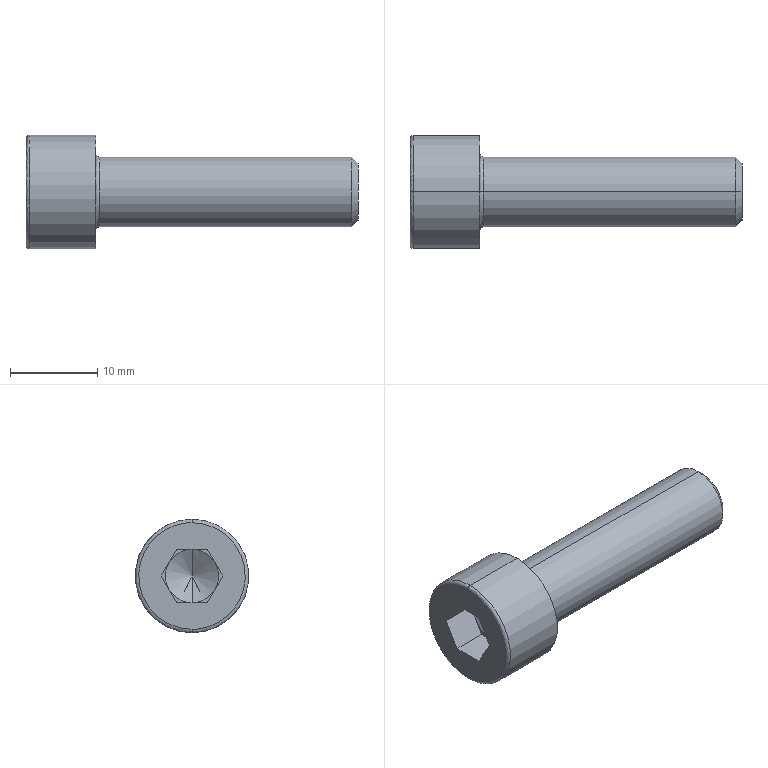Part | SolidWorks | features BaseBody 1 | 1 solid | 27 faces | box 38 x 13 x 13 mm | volume 2418 mm3 | plane 15 | spline 4 | cylinder 4 | cone 4 | commonest cylinder face diameters 8 x2 13 x2
STEP:
#1=CARTESIAN_POINT('',(8.,0.,4.4));
#2=VERTEX_POINT('',#1);
#3=CARTESIAN_POINT('',(8.,0.,-4.4));
#4=VERTEX_POINT('',#3);
#5=CARTESIAN_POINT('',(8.,0.,4.4));
#6=CARTESIAN_POINT('',(8.,0.2797,4.4));
#7=CARTESIAN_POINT('',(8.,0.6919,4.361));
#8=CARTESIAN_POINT('',(8.,1.16,4.249));
#9=CARTESIAN_POINT('',(8.,1.391,4.176));
#10=CARTESIAN_POINT('',(8.,1.489,4.141));
#11=CARTESIAN_POINT('',(8.,1.554,4.116));
#12=CARTESIAN_POINT('',(8.,1.585,4.105));
#13=CARTESIAN_POINT('',(8.,1.758,4.036));
#14=CARTESIAN_POINT('',(8.,1.96,3.944));
#15=CARTESIAN_POINT('',(8.,2.154,3.837));
#16=CARTESIAN_POINT('',(8.,2.282,3.763));
#17=CARTESIAN_POINT('',(8.,2.344,3.724));
#18=CARTESIAN_POINT('',(8.,2.662,3.517));
#19=CARTESIAN_POINT('',(8.,2.897,3.326));
#20=CARTESIAN_POINT('',(8.,3.219,3.004));
#21=CARTESIAN_POINT('',(8.,3.37,2.836));
#22=CARTESIAN_POINT('',(8.,3.509,2.656));
#23=CARTESIAN_POINT('',(8.,3.598,2.534));
#24=CARTESIAN_POINT('',(8.,3.642,2.47));
#25=CARTESIAN_POINT('',(8.,3.764,2.283));
#26=CARTESIAN_POINT('',(8.,3.876,2.092));
#27=CARTESIAN_POINT('',(8.,3.989,1.859));
#28=CARTESIAN_POINT('',(8.,4.042,1.74));
#29=CARTESIAN_POINT('',(8.,4.063,1.689));
#30=CARTESIAN_POINT('',(8.,4.077,1.654));
#31=CARTESIAN_POINT('',(8.,4.085,1.636));
#32=CARTESIAN_POINT('',(8.,4.297,1.1));
#33=CARTESIAN_POINT('',(8.,4.4,0.5592));
#34=CARTESIAN_POINT('',(8.,4.4,-0.2796));
#35=CARTESIAN_POINT('',(8.,4.361,-0.6917));
#36=CARTESIAN_POINT('',(8.,4.249,-1.16));
#37=CARTESIAN_POINT('',(8.,4.176,-1.391));
#38=CARTESIAN_POINT('',(8.,4.141,-1.489));
#39=CARTESIAN_POINT('',(8.,4.116,-1.554));
#40=CARTESIAN_POINT('',(8.,4.105,-1.585));
#41=CARTESIAN_POINT('',(8.,4.036,-1.758));
#42=CARTESIAN_POINT('',(8.,3.944,-1.96));
#43=CARTESIAN_POINT('',(8.,3.837,-2.154));
#44=CARTESIAN_POINT('',(8.,3.763,-2.282));
#45=CARTESIAN_POINT('',(8.,3.724,-2.344));
#46=CARTESIAN_POINT('',(8.,3.517,-2.662));
#47=CARTESIAN_POINT('',(8.,3.326,-2.897));
#48=CARTESIAN_POINT('',(8.,3.004,-3.219));
#49=CARTESIAN_POINT('',(8.,2.836,-3.37));
#50=CARTESIAN_POINT('',(8.,2.656,-3.509));
#51=CARTESIAN_POINT('',(8.,2.534,-3.598));
#52=CARTESIAN_POINT('',(8.,2.47,-3.642));
#53=CARTESIAN_POINT('',(8.,2.283,-3.764));
#54=CARTESIAN_POINT('',(8.,2.092,-3.876));
#55=CARTESIAN_POINT('',(8.,1.859,-3.989));
#56=CARTESIAN_POINT('',(8.,1.74,-4.042));
#57=CARTESIAN_POINT('',(8.,1.689,-4.063));
#58=CARTESIAN_POINT('',(8.,1.654,-4.077));
#59=CARTESIAN_POINT('',(8.,1.636,-4.085));
#60=CARTESIAN_POINT('',(8.,1.1,-4.297));
#61=CARTESIAN_POINT('',(8.,0.5597,-4.4));
#62=CARTESIAN_POINT('',(8.,0.,-4.4));
#63=B_SPLINE_CURVE_WITH_KNOTS('',3,(#5,#6,#7,#8,#9,#10,#11,#12,#13,#14,#15,#16,#17,#18,#19,#20,#21,#22,#23,#24,#25,#26,#27,#28,#29,#30,#31,#32,#33,#34,#35,#36,#37,#38,#39,#40,#41,#42,#43,#44,#45,#46,#47,#48,#49,#50,#51,#52,#53,#54,#55,#56,#57,#58,#59,#60,#61,#62),.UNSPECIFIED.,.F.,.F.,(4,1,1,1,2,2,1,2,2,2,1,2,2,1,1,1,2,2,2,1,1,1,2,2,1,2,2,2,1,2,2,1,1,1,2,2,4),(0.,0.0625,0.09375,0.1094,0.1172,0.125,0.1563,0.1719,0.1875,0.25,0.2813,0.2969,0.3125,0.3438,0.3594,0.3672,0.3711,0.375,0.5,0.5625,0.5938,0.6094,0.6172,0.625,0.6563,0.6719,0.6875,0.75,0.7813,0.7969,0.8125,0.8438,0.8594,0.8672,0.8711,0.875,1.),.UNSPECIFIED.);
#64=EDGE_CURVE('',#2,#4,#63,.T.);
#65=ORIENTED_EDGE('',*,*,#64,.F.);
#66=CARTESIAN_POINT('',(8.4,0.,4.));
#67=VERTEX_POINT('',#66);
#68=CARTESIAN_POINT('',(8.4,0.,4.4));
#69=DIRECTION('',(0.,-1.,0.));
#70=DIRECTION('',(0.,0.,1.));
#71=AXIS2_PLACEMENT_3D('',#68,#69,#70);
#72=CIRCLE('',#71,0.4);
#73=EDGE_CURVE('',#2,#67,#72,.T.);
#74=ORIENTED_EDGE('',*,*,#73,.T.);
#75=CARTESIAN_POINT('',(8.4,0.,-4.));
#76=VERTEX_POINT('',#75);
#77=CARTESIAN_POINT('',(8.4,0.,0.));
#78=DIRECTION('',(1.,0.,0.));
#79=DIRECTION('',(0.,0.,1.));
#80=AXIS2_PLACEMENT_3D('',#77,#78,#79);
#81=CIRCLE('',#80,4.);
#82=EDGE_CURVE('',#76,#67,#81,.T.);
#83=ORIENTED_EDGE('',*,*,#82,.F.);
#84=CARTESIAN_POINT('',(8.4,0.,-4.4));
#85=DIRECTION('',(0.,1.,0.));
#86=DIRECTION('',(0.,0.,-1.));
#87=AXIS2_PLACEMENT_3D('',#84,#85,#86);
#88=CIRCLE('',#87,0.4);
#89=EDGE_CURVE('',#4,#76,#88,.T.);
#90=ORIENTED_EDGE('',*,*,#89,.F.);
#91=EDGE_LOOP('',(#65,#74,#83,#90));
#92=FACE_OUTER_BOUND('',#91,.T.);
#93=CARTESIAN_POINT('',(8.,0.,-4.4));
#94=CARTESIAN_POINT('',(8.,8.8,-4.4));
#95=CARTESIAN_POINT('',(8.,8.8,4.4));
#96=CARTESIAN_POINT('',(8.,0.,4.4));
#97=CARTESIAN_POINT('',(8.,0.,-4.166));
#98=CARTESIAN_POINT('',(8.,8.331,-4.166));
#99=CARTESIAN_POINT('',(8.,8.331,4.166));
#100=CARTESIAN_POINT('',(8.,0.,4.166));
#101=CARTESIAN_POINT('',(8.166,0.,-4.));
#102=CARTESIAN_POINT('',(8.166,8.,-4.));
#103=CARTESIAN_POINT('',(8.166,8.,4.));
#104=CARTESIAN_POINT('',(8.166,0.,4.));
#105=CARTESIAN_POINT('',(8.4,0.,-4.));
#106=CARTESIAN_POINT('',(8.4,8.,-4.));
#107=CARTESIAN_POINT('',(8.4,8.,4.));
#108=CARTESIAN_POINT('',(8.4,0.,4.));
#109=(BOUNDED_SURFACE()B_SPLINE_SURFACE(3,3,((#93,#94,#95,#96),(#97,#98,#99,#100),(#101,#102,#103,#104),(#105,#106,#107,#108)),.UNSPECIFIED.,.F.,.F.,.F.)B_SPLINE_SURFACE_WITH_KNOTS((4,4),(4,4),(0.,1.),(0.,1.),.UNSPECIFIED.)GEOMETRIC_REPRESENTATION_ITEM()RATIONAL_B_SPLINE_SURFACE(((1.,0.3333,0.3333,1.),(0.8047,0.2682,0.2682,0.8047),(0.8047,0.2682,0.2682,0.8047),(1.,0.3333,0.3333,1.)))REPRESENTATION_ITEM('')SURFACE());
#110=ADVANCED_FACE('',(#92),#109,.F.);
#111=CARTESIAN_POINT('',(0.,0.,6.1));
#112=VERTEX_POINT('',#111);
#113=CARTESIAN_POINT('',(0.,0.,-6.1));
#114=VERTEX_POINT('',#113);
#115=CARTESIAN_POINT('',(0.,0.,6.1));
#116=CARTESIAN_POINT('',(0.,-12.2,6.1));
#117=CARTESIAN_POINT('',(0.,-12.2,-6.1));
#118=CARTESIAN_POINT('',(0.,0.,-6.1));
#119=(BOUNDED_CURVE()B_SPLINE_CURVE(3,(#115,#116,#117,#118),.UNSPECIFIED.,.F.,.T.)B_SPLINE_CURVE_WITH_KNOTS((4,4),(0.,1.),.UNSPECIFIED.)CURVE()GEOMETRIC_REPRESENTATION_ITEM()RATIONAL_B_SPLINE_CURVE((1.,0.3333,0.3333,1.))REPRESENTATION_ITEM(''));
#120=EDGE_CURVE('',#112,#114,#119,.T.);
#121=ORIENTED_EDGE('',*,*,#120,.T.);
#122=CARTESIAN_POINT('',(0.4,0.,-6.5));
#123=VERTEX_POINT('',#122);
#124=CARTESIAN_POINT('',(0.4,0.,-6.1));
#125=DIRECTION('',(0.,-1.,0.));
#126=DIRECTION('',(0.,0.,-1.));
#127=AXIS2_PLACEMENT_3D('',#124,#125,#126);
#128=CIRCLE('',#127,0.4);
#129=EDGE_CURVE('',#114,#123,#128,.T.);
#130=ORIENTED_EDGE('',*,*,#129,.T.);
#131=CARTESIAN_POINT('',(0.4,0.,6.5));
#132=VERTEX_POINT('',#131);
#133=CARTESIAN_POINT('',(0.4,0.,0.));
#134=DIRECTION('',(1.,0.,0.));
#135=DIRECTION('',(0.,0.,1.));
#136=AXIS2_PLACEMENT_3D('',#133,#134,#135);
#137=CIRCLE('',#136,6.5);
#138=EDGE_CURVE('',#132,#123,#137,.T.);
#139=ORIENTED_EDGE('',*,*,#138,.F.);
#140=CARTESIAN_POINT('',(0.4,0.,6.1));
#141=DIRECTION('',(0.,1.,0.));
#142=DIRECTION('',(0.,0.,1.));
#143=AXIS2_PLACEMENT_3D('',#140,#141,#142);
#144=CIRCLE('',#143,0.4);
#145=EDGE_CURVE('',#112,#132,#144,.T.);
#146=ORIENTED_EDGE('',*,*,#145,.F.);
#147=EDGE_LOOP('',(#121,#130,#139,#146));
#148=FACE_OUTER_BOUND('',#147,.T.);
#149=CARTESIAN_POINT('',(0.,0.,-6.1));
#150=CARTESIAN_POINT('',(0.,-12.2,-6.1));
#151=CARTESIAN_POINT('',(0.,-12.2,6.1));
#152=CARTESIAN_POINT('',(0.,0.,6.1));
#153=CARTESIAN_POINT('',(0.,0.,-6.334));
#154=CARTESIAN_POINT('',(0.,-12.669,-6.334));
#155=CARTESIAN_POINT('',(0.,-12.669,6.334));
#156=CARTESIAN_POINT('',(0.,0.,6.334));
#157=CARTESIAN_POINT('',(0.1657,0.,-6.5));
#158=CARTESIAN_POINT('',(0.1657,-13.,-6.5));
#159=CARTESIAN_POINT('',(0.1657,-13.,6.5));
#160=CARTESIAN_POINT('',(0.1657,0.,6.5));
#161=CARTESIAN_POINT('',(0.4,0.,-6.5));
#162=CARTESIAN_POINT('',(0.4,-13.,-6.5));
#163=CARTESIAN_POINT('',(0.4,-13.,6.5));
#164=CARTESIAN_POINT('',(0.4,0.,6.5));
#165=(BOUNDED_SURFACE()B_SPLINE_SURFACE(3,3,((#149,#150,#151,#152),(#153,#154,#155,#156),(#157,#158,#159,#160),(#161,#162,#163,#164)),.UNSPECIFIED.,.F.,.F.,.T.)B_SPLINE_SURFACE_WITH_KNOTS((4,4),(4,4),(0.,1.),(0.,1.),.UNSPECIFIED.)GEOMETRIC_REPRESENTATION_ITEM()RATIONAL_B_SPLINE_SURFACE(((1.,0.3333,0.3333,1.),(0.8047,0.2682,0.2682,0.8047),(0.8047,0.2682,0.2682,0.8047),(1.,0.3333,0.3333,1.)))REPRESENTATION_ITEM('')SURFACE());
#166=ADVANCED_FACE('',(#148),#165,.T.);
#167=CARTESIAN_POINT('',(37.31,0.,4.));
#168=VERTEX_POINT('',#167);
#169=CARTESIAN_POINT('',(37.31,0.,-4.));
#170=VERTEX_POINT('',#169);
#171=CARTESIAN_POINT('',(37.31,0.,0.));
#172=DIRECTION('',(-1.,0.,0.));
#173=DIRECTION('',(0.,0.,1.));
#174=AXIS2_PLACEMENT_3D('',#171,#172,#173);
#175=CIRCLE('',#174,4.);
#176=EDGE_CURVE('',#168,#170,#175,.T.);
#177=ORIENTED_EDGE('',*,*,#176,.T.);
#178=CARTESIAN_POINT('',(-31.75,0.,-4.));
#179=DIRECTION('',(-1.,0.,0.));
#180=VECTOR('',#179,1000.);
#181=LINE('',#178,#180);
#182=EDGE_CURVE('',#170,#76,#181,.T.);
#183=ORIENTED_EDGE('',*,*,#182,.T.);
#184=ORIENTED_EDGE('',*,*,#82,.T.);
#185=CARTESIAN_POINT('',(-31.75,0.,4.));
#186=DIRECTION('',(-1.,0.,0.));
#187=VECTOR('',#186,1000.);
#188=LINE('',#185,#187);
#189=EDGE_CURVE('',#168,#67,#188,.T.);
#190=ORIENTED_EDGE('',*,*,#189,.F.);
#191=EDGE_LOOP('',(#177,#183,#184,#190));
#192=FACE_OUTER_BOUND('',#191,.T.);
#193=CARTESIAN_POINT('',(-31.75,0.,0.));
#194=DIRECTION('',(-1.,0.,0.));
#195=DIRECTION('',(0.,0.,1.));
#196=AXIS2_PLACEMENT_3D('',#193,#194,#195);
#197=CYLINDRICAL_SURFACE('',#196,4.);
#198=ADVANCED_FACE('',(#192),#197,.T.);
#199=CARTESIAN_POINT('',(38.,0.,3.309));
#200=VERTEX_POINT('',#199);
#201=CARTESIAN_POINT('',(38.,0.,-3.309));
#202=VERTEX_POINT('',#201);
#203=CARTESIAN_POINT('',(38.,0.,0.));
#204=DIRECTION('',(-1.,0.,0.));
#205=DIRECTION('',(0.,0.,1.));
#206=AXIS2_PLACEMENT_3D('',#203,#204,#205);
#207=CIRCLE('',#206,3.309);
#208=EDGE_CURVE('',#200,#202,#207,.T.);
#209=ORIENTED_EDGE('',*,*,#208,.T.);
#210=CARTESIAN_POINT('',(37.31,0.,-4.));
#211=DIRECTION('',(-0.7071,0.,-0.7071));
#212=VECTOR('',#211,1000.);
#213=LINE('',#210,#212);
#214=EDGE_CURVE('',#202,#170,#213,.T.);
#215=ORIENTED_EDGE('',*,*,#214,.T.);
#216=ORIENTED_EDGE('',*,*,#176,.F.);
#217=CARTESIAN_POINT('',(37.31,0.,4.));
#218=DIRECTION('',(-0.7071,0.,0.7071));
#219=VECTOR('',#218,1000.);
#220=LINE('',#217,#219);
#221=EDGE_CURVE('',#200,#168,#220,.T.);
#222=ORIENTED_EDGE('',*,*,#221,.F.);
#223=EDGE_LOOP('',(#209,#215,#216,#222));
#224=FACE_OUTER_BOUND('',#223,.T.);
#225=CARTESIAN_POINT('',(37.31,0.,0.));
#226=DIRECTION('',(-1.,0.,0.));
#227=DIRECTION('',(0.,0.,1.));
#228=AXIS2_PLACEMENT_3D('',#225,#226,#227);
#229=CONICAL_SURFACE('',#228,4.,0.7854);
#230=ADVANCED_FACE('',(#224),#229,.T.);
#231=CARTESIAN_POINT('',(8.,0.,-6.5));
#232=VERTEX_POINT('',#231);
#233=CARTESIAN_POINT('',(8.,0.,6.5));
#234=VERTEX_POINT('',#233);
#235=CARTESIAN_POINT('',(8.,0.,0.));
#236=DIRECTION('',(1.,0.,0.));
#237=DIRECTION('',(0.,0.,1.));
#238=AXIS2_PLACEMENT_3D('',#235,#236,#237);
#239=CIRCLE('',#238,6.5);
#240=EDGE_CURVE('',#232,#234,#239,.T.);
#241=ORIENTED_EDGE('',*,*,#240,.F.);
#242=CARTESIAN_POINT('',(-31.75,0.,-6.5));
#243=DIRECTION('',(-1.,0.,0.));
#244=VECTOR('',#243,1000.);
#245=LINE('',#242,#244);
#246=EDGE_CURVE('',#232,#123,#245,.T.);
#247=ORIENTED_EDGE('',*,*,#246,.T.);
#248=CARTESIAN_POINT('',(0.4,0.,0.));
#249=DIRECTION('',(1.,0.,0.));
#250=DIRECTION('',(0.,0.,1.));
#251=AXIS2_PLACEMENT_3D('',#248,#249,#250);
#252=CIRCLE('',#251,6.5);
#253=EDGE_CURVE('',#123,#132,#252,.T.);
#254=ORIENTED_EDGE('',*,*,#253,.T.);
#255=CARTESIAN_POINT('',(-31.75,0.,6.5));
#256=DIRECTION('',(-1.,0.,0.));
#257=VECTOR('',#256,1000.);
#258=LINE('',#255,#257);
#259=EDGE_CURVE('',#234,#132,#258,.T.);
#260=ORIENTED_EDGE('',*,*,#259,.F.);
#261=EDGE_LOOP('',(#241,#247,#254,#260));
#262=FACE_OUTER_BOUND('',#261,.T.);
#263=CARTESIAN_POINT('',(-31.75,0.,0.));
#264=DIRECTION('',(-1.,0.,0.));
#265=DIRECTION('',(0.,0.,1.));
#266=AXIS2_PLACEMENT_3D('',#263,#264,#265);
#267=CYLINDRICAL_SURFACE('',#266,6.5);
#268=ADVANCED_FACE('',(#262),#267,.T.);
#269=CARTESIAN_POINT('',(5.759,0.,0.));
#270=VERTEX_POINT('',#269);
#271=CARTESIAN_POINT('',(4.,0.,3.047));
#272=VERTEX_POINT('',#271);
#273=CARTESIAN_POINT('',(4.,0.,3.047));
#274=DIRECTION('',(-0.5,0.,0.866));
#275=VECTOR('',#274,1000.);
#276=LINE('',#273,#275);
#277=EDGE_CURVE('',#270,#272,#276,.T.);
#278=ORIENTED_EDGE('',*,*,#277,.F.);
#279=CARTESIAN_POINT('',(4.,0.,-3.047));
#280=VERTEX_POINT('',#279);
#281=CARTESIAN_POINT('',(4.,0.,-3.047));
#282=DIRECTION('',(-0.5,0.,-0.866));
#283=VECTOR('',#282,1000.);
#284=LINE('',#281,#283);
#285=EDGE_CURVE('',#270,#280,#284,.T.);
#286=ORIENTED_EDGE('',*,*,#285,.T.);
#287=CARTESIAN_POINT('',(4.,-2.639,-1.524));
#288=VERTEX_POINT('',#287);
#289=CARTESIAN_POINT('',(4.,0.,0.));
#290=DIRECTION('',(-1.,0.,0.));
#291=DIRECTION('',(0.,0.,1.));
#292=AXIS2_PLACEMENT_3D('',#289,#290,#291);
#293=CIRCLE('',#292,3.047);
#294=EDGE_CURVE('',#280,#288,#293,.T.);
#295=ORIENTED_EDGE('',*,*,#294,.T.);
#296=CARTESIAN_POINT('',(4.,-2.639,1.524));
#297=VERTEX_POINT('',#296);
#298=CARTESIAN_POINT('',(4.,0.,0.));
#299=DIRECTION('',(-1.,0.,0.));
#300=DIRECTION('',(0.,0.,1.));
#301=AXIS2_PLACEMENT_3D('',#298,#299,#300);
#302=CIRCLE('',#301,3.047);
#303=EDGE_CURVE('',#288,#297,#302,.T.);
#304=ORIENTED_EDGE('',*,*,#303,.T.);
#305=CARTESIAN_POINT('',(4.,0.,0.));
#306=DIRECTION('',(-1.,0.,0.));
#307=DIRECTION('',(0.,0.,1.));
#308=AXIS2_PLACEMENT_3D('',#305,#306,#307);
#309=CIRCLE('',#308,3.047);
#310=EDGE_CURVE('',#297,#272,#309,.T.);
#311=ORIENTED_EDGE('',*,*,#310,.T.);
#312=EDGE_LOOP('',(#278,#286,#295,#304,#311));
#313=FACE_OUTER_BOUND('',#312,.T.);
#314=CARTESIAN_POINT('',(4.,0.,0.));
#315=DIRECTION('',(-1.,0.,0.));
#316=DIRECTION('',(0.,0.,1.));
#317=AXIS2_PLACEMENT_3D('',#314,#315,#316);
#318=CONICAL_SURFACE('',#317,3.047,1.047);
#319=ADVANCED_FACE('',(#313),#318,.F.);
#320=ORIENTED_EDGE('',*,*,#182,.F.);
#321=CARTESIAN_POINT('',(37.31,0.,0.));
#322=DIRECTION('',(-1.,0.,0.));
#323=DIRECTION('',(0.,0.,1.));
#324=AXIS2_PLACEMENT_3D('',#321,#322,#323);
#325=CIRCLE('',#324,4.);
#326=EDGE_CURVE('',#170,#168,#325,.T.);
#327=ORIENTED_EDGE('',*,*,#326,.T.);
#328=ORIENTED_EDGE('',*,*,#189,.T.);
#329=CARTESIAN_POINT('',(8.4,0.,0.));
#330=DIRECTION('',(1.,0.,0.));
#331=DIRECTION('',(0.,0.,1.));
#332=AXIS2_PLACEMENT_3D('',#329,#330,#331);
#333=CIRCLE('',#332,4.);
#334=EDGE_CURVE('',#67,#76,#333,.T.);
#335=ORIENTED_EDGE('',*,*,#334,.T.);
#336=EDGE_LOOP('',(#320,#327,#328,#335));
#337=FACE_OUTER_BOUND('',#336,.T.);
#338=CARTESIAN_POINT('',(-31.75,0.,0.));
#339=DIRECTION('',(-1.,0.,0.));
#340=DIRECTION('',(0.,0.,1.));
#341=AXIS2_PLACEMENT_3D('',#338,#339,#340);
#342=CYLINDRICAL_SURFACE('',#341,4.);
#343=ADVANCED_FACE('',(#337),#342,.T.);
#344=ORIENTED_EDGE('',*,*,#73,.F.);
#345=CARTESIAN_POINT('',(8.,0.,-4.4));
#346=CARTESIAN_POINT('',(8.,-0.2797,-4.4));
#347=CARTESIAN_POINT('',(8.,-0.6919,-4.361));
#348=CARTESIAN_POINT('',(8.,-1.16,-4.249));
#349=CARTESIAN_POINT('',(8.,-1.391,-4.176));
#350=CARTESIAN_POINT('',(8.,-1.489,-4.141));
#351=CARTESIAN_POINT('',(8.,-1.554,-4.116));
#352=CARTESIAN_POINT('',(8.,-1.585,-4.105));
#353=CARTESIAN_POINT('',(8.,-1.758,-4.036));
#354=CARTESIAN_POINT('',(8.,-1.96,-3.944));
#355=CARTESIAN_POINT('',(8.,-2.154,-3.837));
#356=CARTESIAN_POINT('',(8.,-2.282,-3.763));
#357=CARTESIAN_POINT('',(8.,-2.344,-3.724));
#358=CARTESIAN_POINT('',(8.,-2.662,-3.517));
#359=CARTESIAN_POINT('',(8.,-2.897,-3.326));
#360=CARTESIAN_POINT('',(8.,-3.219,-3.004));
#361=CARTESIAN_POINT('',(8.,-3.37,-2.836));
#362=CARTESIAN_POINT('',(8.,-3.509,-2.656));
#363=CARTESIAN_POINT('',(8.,-3.598,-2.534));
#364=CARTESIAN_POINT('',(8.,-3.642,-2.47));
#365=CARTESIAN_POINT('',(8.,-3.764,-2.283));
#366=CARTESIAN_POINT('',(8.,-3.876,-2.092));
#367=CARTESIAN_POINT('',(8.,-3.989,-1.859));
#368=CARTESIAN_POINT('',(8.,-4.042,-1.74));
#369=CARTESIAN_POINT('',(8.,-4.063,-1.689));
#370=CARTESIAN_POINT('',(8.,-4.077,-1.654));
#371=CARTESIAN_POINT('',(8.,-4.085,-1.636));
#372=CARTESIAN_POINT('',(8.,-4.297,-1.1));
#373=CARTESIAN_POINT('',(8.,-4.4,-0.5592));
#374=CARTESIAN_POINT('',(8.,-4.4,0.2796));
#375=CARTESIAN_POINT('',(8.,-4.361,0.6917));
#376=CARTESIAN_POINT('',(8.,-4.249,1.16));
#377=CARTESIAN_POINT('',(8.,-4.176,1.391));
#378=CARTESIAN_POINT('',(8.,-4.141,1.489));
#379=CARTESIAN_POINT('',(8.,-4.116,1.554));
#380=CARTESIAN_POINT('',(8.,-4.105,1.585));
#381=CARTESIAN_POINT('',(8.,-4.036,1.758));
#382=CARTESIAN_POINT('',(8.,-3.944,1.96));
#383=CARTESIAN_POINT('',(8.,-3.837,2.154));
#384=CARTESIAN_POINT('',(8.,-3.763,2.282));
#385=CARTESIAN_POINT('',(8.,-3.724,2.344));
#386=CARTESIAN_POINT('',(8.,-3.517,2.662));
#387=CARTESIAN_POINT('',(8.,-3.326,2.897));
#388=CARTESIAN_POINT('',(8.,-3.004,3.219));
#389=CARTESIAN_POINT('',(8.,-2.836,3.37));
#390=CARTESIAN_POINT('',(8.,-2.656,3.509));
#391=CARTESIAN_POINT('',(8.,-2.534,3.598));
#392=CARTESIAN_POINT('',(8.,-2.47,3.642));
#393=CARTESIAN_POINT('',(8.,-2.283,3.764));
#394=CARTESIAN_POINT('',(8.,-2.092,3.876));
#395=CARTESIAN_POINT('',(8.,-1.859,3.989));
#396=CARTESIAN_POINT('',(8.,-1.74,4.042));
#397=CARTESIAN_POINT('',(8.,-1.689,4.063));
#398=CARTESIAN_POINT('',(8.,-1.654,4.077));
#399=CARTESIAN_POINT('',(8.,-1.636,4.085));
#400=CARTESIAN_POINT('',(8.,-1.1,4.297));
#401=CARTESIAN_POINT('',(8.,-0.5597,4.4));
#402=CARTESIAN_POINT('',(8.,0.,4.4));
#403=B_SPLINE_CURVE_WITH_KNOTS('',3,(#345,#346,#347,#348,#349,#350,#351,#352,#353,#354,#355,#356,#357,#358,#359,#360,#361,#362,#363,#364,#365,#366,#367,#368,#369,#370,#371,#372,#373,#374,#375,#376,#377,#378,#379,#380,#381,#382,#383,#384,#385,#386,#387,#388,#389,#390,#391,#392,#393,#394,#395,#396,#397,#398,#399,#400,#401,#402),.UNSPECIFIED.,.F.,.F.,(4,1,1,1,2,2,1,2,2,2,1,2,2,1,1,1,2,2,2,1,1,1,2,2,1,2,2,2,1,2,2,1,1,1,2,2,4),(0.,0.0625,0.09375,0.1094,0.1172,0.125,0.1562,0.1719,0.1875,0.25,0.2812,0.2969,0.3125,0.3437,0.3594,0.3672,0.3711,0.375,0.5,0.5625,0.5937,0.6094,0.6172,0.625,0.6562,0.6719,0.6875,0.75,0.7812,0.7969,0.8125,0.8437,0.8594,0.8672,0.8711,0.875,1.),.UNSPECIFIED.);
#404=EDGE_CURVE('',#4,#2,#403,.T.);
#405=ORIENTED_EDGE('',*,*,#404,.F.);
#406=ORIENTED_EDGE('',*,*,#89,.T.);
#407=ORIENTED_EDGE('',*,*,#334,.F.);
#408=EDGE_LOOP('',(#344,#405,#406,#407));
#409=FACE_OUTER_BOUND('',#408,.T.);
#410=CARTESIAN_POINT('',(8.,0.,4.4));
#411=CARTESIAN_POINT('',(8.,-8.8,4.4));
#412=CARTESIAN_POINT('',(8.,-8.8,-4.4));
#413=CARTESIAN_POINT('',(8.,0.,-4.4));
#414=CARTESIAN_POINT('',(8.,0.,4.166));
#415=CARTESIAN_POINT('',(8.,-8.331,4.166));
#416=CARTESIAN_POINT('',(8.,-8.331,-4.166));
#417=CARTESIAN_POINT('',(8.,0.,-4.166));
#418=CARTESIAN_POINT('',(8.166,0.,4.));
#419=CARTESIAN_POINT('',(8.166,-8.,4.));
#420=CARTESIAN_POINT('',(8.166,-8.,-4.));
#421=CARTESIAN_POINT('',(8.166,0.,-4.));
#422=CARTESIAN_POINT('',(8.4,0.,4.));
#423=CARTESIAN_POINT('',(8.4,-8.,4.));
#424=CARTESIAN_POINT('',(8.4,-8.,-4.));
#425=CARTESIAN_POINT('',(8.4,0.,-4.));
#426=(BOUNDED_SURFACE()B_SPLINE_SURFACE(3,3,((#410,#411,#412,#413),(#414,#415,#416,#417),(#418,#419,#420,#421),(#422,#423,#424,#425)),.UNSPECIFIED.,.F.,.F.,.T.)B_SPLINE_SURFACE_WITH_KNOTS((4,4),(4,4),(0.,1.),(0.,1.),.UNSPECIFIED.)GEOMETRIC_REPRESENTATION_ITEM()RATIONAL_B_SPLINE_SURFACE(((1.,0.3333,0.3333,1.),(0.8047,0.2682,0.2682,0.8047),(0.8047,0.2682,0.2682,0.8047),(1.,0.3333,0.3333,1.)))REPRESENTATION_ITEM('')SURFACE());
#427=ADVANCED_FACE('',(#409),#426,.F.);
#428=ORIENTED_EDGE('',*,*,#214,.F.);
#429=CARTESIAN_POINT('',(38.,0.,0.));
#430=DIRECTION('',(-1.,0.,0.));
#431=DIRECTION('',(0.,0.,1.));
#432=AXIS2_PLACEMENT_3D('',#429,#430,#431);
#433=CIRCLE('',#432,3.309);
#434=EDGE_CURVE('',#202,#200,#433,.T.);
#435=ORIENTED_EDGE('',*,*,#434,.T.);
#436=ORIENTED_EDGE('',*,*,#221,.T.);
#437=ORIENTED_EDGE('',*,*,#326,.F.);
#438=EDGE_LOOP('',(#428,#435,#436,#437));
#439=FACE_OUTER_BOUND('',#438,.T.);
#440=CARTESIAN_POINT('',(37.31,0.,0.));
#441=DIRECTION('',(-1.,0.,0.));
#442=DIRECTION('',(0.,0.,1.));
#443=AXIS2_PLACEMENT_3D('',#440,#441,#442);
#444=CONICAL_SURFACE('',#443,4.,0.7854);
#445=ADVANCED_FACE('',(#439),#444,.T.);
#446=CARTESIAN_POINT('',(8.,0.,0.));
#447=DIRECTION('',(1.,0.,0.));
#448=DIRECTION('',(0.,0.,1.));
#449=AXIS2_PLACEMENT_3D('',#446,#447,#448);
#450=CIRCLE('',#449,6.5);
#451=EDGE_CURVE('',#234,#232,#450,.T.);
#452=ORIENTED_EDGE('',*,*,#451,.T.);
#453=ORIENTED_EDGE('',*,*,#240,.T.);
#454=EDGE_LOOP('',(#452,#453));
#455=FACE_OUTER_BOUND('',#454,.T.);
#456=ORIENTED_EDGE('',*,*,#404,.T.);
#457=ORIENTED_EDGE('',*,*,#64,.T.);
#458=EDGE_LOOP('',(#456,#457));
#459=FACE_BOUND('',#458,.T.);
#460=CARTESIAN_POINT('',(8.,6.5,0.));
#461=DIRECTION('',(1.,0.,0.));
#462=DIRECTION('',(0.,0.,-1.));
#463=AXIS2_PLACEMENT_3D('',#460,#461,#462);
#464=PLANE('',#463);
#465=ADVANCED_FACE('',(#455,#459),#464,.T.);
#466=ORIENTED_EDGE('',*,*,#208,.F.);
#467=ORIENTED_EDGE('',*,*,#434,.F.);
#468=EDGE_LOOP('',(#466,#467));
#469=FACE_OUTER_BOUND('',#468,.T.);
#470=CARTESIAN_POINT('',(38.,3.309,0.));
#471=DIRECTION('',(1.,0.,0.));
#472=DIRECTION('',(0.,0.,-1.));
#473=AXIS2_PLACEMENT_3D('',#470,#471,#472);
#474=PLANE('',#473);
#475=ADVANCED_FACE('',(#469),#474,.T.);
#476=ORIENTED_EDGE('',*,*,#246,.F.);
#477=ORIENTED_EDGE('',*,*,#451,.F.);
#478=ORIENTED_EDGE('',*,*,#259,.T.);
#479=ORIENTED_EDGE('',*,*,#138,.T.);
#480=EDGE_LOOP('',(#476,#477,#478,#479));
#481=FACE_OUTER_BOUND('',#480,.T.);
#482=CARTESIAN_POINT('',(-31.75,0.,0.));
#483=DIRECTION('',(-1.,0.,0.));
#484=DIRECTION('',(0.,0.,1.));
#485=AXIS2_PLACEMENT_3D('',#482,#483,#484);
#486=CYLINDRICAL_SURFACE('',#485,6.5);
#487=ADVANCED_FACE('',(#481),#486,.T.);
#488=ORIENTED_EDGE('',*,*,#129,.F.);
#489=CARTESIAN_POINT('',(0.,0.,-6.1));
#490=CARTESIAN_POINT('',(0.,12.2,-6.1));
#491=CARTESIAN_POINT('',(0.,12.2,6.1));
#492=CARTESIAN_POINT('',(0.,0.,6.1));
#493=(BOUNDED_CURVE()B_SPLINE_CURVE(3,(#489,#490,#491,#492),.UNSPECIFIED.,.F.,.F.)B_SPLINE_CURVE_WITH_KNOTS((4,4),(0.,1.),.UNSPECIFIED.)CURVE()GEOMETRIC_REPRESENTATION_ITEM()RATIONAL_B_SPLINE_CURVE((1.,0.3333,0.3333,1.))REPRESENTATION_ITEM(''));
#494=EDGE_CURVE('',#114,#112,#493,.T.);
#495=ORIENTED_EDGE('',*,*,#494,.T.);
#496=ORIENTED_EDGE('',*,*,#145,.T.);
#497=ORIENTED_EDGE('',*,*,#253,.F.);
#498=EDGE_LOOP('',(#488,#495,#496,#497));
#499=FACE_OUTER_BOUND('',#498,.T.);
#500=CARTESIAN_POINT('',(0.,0.,6.1));
#501=CARTESIAN_POINT('',(0.,12.2,6.1));
#502=CARTESIAN_POINT('',(0.,12.2,-6.1));
#503=CARTESIAN_POINT('',(0.,0.,-6.1));
#504=CARTESIAN_POINT('',(0.,0.,6.334));
#505=CARTESIAN_POINT('',(0.,12.669,6.334));
#506=CARTESIAN_POINT('',(0.,12.669,-6.334));
#507=CARTESIAN_POINT('',(0.,0.,-6.334));
#508=CARTESIAN_POINT('',(0.1657,0.,6.5));
#509=CARTESIAN_POINT('',(0.1657,13.,6.5));
#510=CARTESIAN_POINT('',(0.1657,13.,-6.5));
#511=CARTESIAN_POINT('',(0.1657,0.,-6.5));
#512=CARTESIAN_POINT('',(0.4,0.,6.5));
#513=CARTESIAN_POINT('',(0.4,13.,6.5));
#514=CARTESIAN_POINT('',(0.4,13.,-6.5));
#515=CARTESIAN_POINT('',(0.4,0.,-6.5));
#516=(BOUNDED_SURFACE()B_SPLINE_SURFACE(3,3,((#500,#501,#502,#503),(#504,#505,#506,#507),(#508,#509,#510,#511),(#512,#513,#514,#515)),.UNSPECIFIED.,.F.,.F.,.F.)B_SPLINE_SURFACE_WITH_KNOTS((4,4),(4,4),(0.,1.),(0.,1.),.UNSPECIFIED.)GEOMETRIC_REPRESENTATION_ITEM()RATIONAL_B_SPLINE_SURFACE(((1.,0.3333,0.3333,1.),(0.8047,0.2682,0.2682,0.8047),(0.8047,0.2682,0.2682,0.8047),(1.,0.3333,0.3333,1.)))REPRESENTATION_ITEM('')SURFACE());
#517=ADVANCED_FACE('',(#499),#516,.T.);
#518=ORIENTED_EDGE('',*,*,#494,.F.);
#519=ORIENTED_EDGE('',*,*,#120,.F.);
#520=EDGE_LOOP('',(#518,#519));
#521=FACE_OUTER_BOUND('',#520,.T.);
#522=CARTESIAN_POINT('',(0.,-1.759,-3.048));
#523=VERTEX_POINT('',#522);
#524=CARTESIAN_POINT('',(0.,1.759,-3.048));
#525=VERTEX_POINT('',#524);
#526=CARTESIAN_POINT('',(0.,0.,-3.048));
#527=DIRECTION('',(0.,1.,0.));
#528=VECTOR('',#527,1000.);
#529=LINE('',#526,#528);
#530=EDGE_CURVE('',#523,#525,#529,.T.);
#531=ORIENTED_EDGE('',*,*,#530,.T.);
#532=CARTESIAN_POINT('',(0.,3.519,0.));
#533=VERTEX_POINT('',#532);
#534=CARTESIAN_POINT('',(0.,1.759,-3.048));
#535=DIRECTION('',(0.,0.5,0.866));
#536=VECTOR('',#535,1000.);
#537=LINE('',#534,#536);
#538=EDGE_CURVE('',#525,#533,#537,.T.);
#539=ORIENTED_EDGE('',*,*,#538,.T.);
#540=CARTESIAN_POINT('',(0.,1.759,3.047));
#541=VERTEX_POINT('',#540);
#542=CARTESIAN_POINT('',(0.,3.519,0.));
#543=DIRECTION('',(0.,-0.5,0.866));
#544=VECTOR('',#543,1000.);
#545=LINE('',#542,#544);
#546=EDGE_CURVE('',#533,#541,#545,.T.);
#547=ORIENTED_EDGE('',*,*,#546,.T.);
#548=CARTESIAN_POINT('',(0.,-1.759,3.047));
#549=VERTEX_POINT('',#548);
#550=CARTESIAN_POINT('',(0.,0.,3.047));
#551=DIRECTION('',(0.,-1.,0.));
#552=VECTOR('',#551,1000.);
#553=LINE('',#550,#552);
#554=EDGE_CURVE('',#541,#549,#553,.T.);
#555=ORIENTED_EDGE('',*,*,#554,.T.);
#556=CARTESIAN_POINT('',(0.,-3.519,0.));
#557=VERTEX_POINT('',#556);
#558=CARTESIAN_POINT('',(0.,-1.759,3.047));
#559=DIRECTION('',(0.,-0.5,-0.866));
#560=VECTOR('',#559,1000.);
#561=LINE('',#558,#560);
#562=EDGE_CURVE('',#549,#557,#561,.T.);
#563=ORIENTED_EDGE('',*,*,#562,.T.);
#564=CARTESIAN_POINT('',(0.,-3.519,0.));
#565=DIRECTION('',(0.,0.5,-0.866));
#566=VECTOR('',#565,1000.);
#567=LINE('',#564,#566);
#568=EDGE_CURVE('',#557,#523,#567,.T.);
#569=ORIENTED_EDGE('',*,*,#568,.T.);
#570=EDGE_LOOP('',(#531,#539,#547,#555,#563,#569));
#571=FACE_BOUND('',#570,.T.);
#572=CARTESIAN_POINT('',(0.,0.,0.));
#573=DIRECTION('',(-1.,0.,0.));
#574=DIRECTION('',(0.,0.,1.));
#575=AXIS2_PLACEMENT_3D('',#572,#573,#574);
#576=PLANE('',#575);
#577=ADVANCED_FACE('',(#521,#571),#576,.T.);
#578=CARTESIAN_POINT('',(4.,1.759,-3.048));
#579=VERTEX_POINT('',#578);
#580=CARTESIAN_POINT('',(4.,1.759,-3.048));
#581=DIRECTION('',(-1.,0.,0.));
#582=VECTOR('',#581,1000.);
#583=LINE('',#580,#582);
#584=EDGE_CURVE('',#579,#525,#583,.T.);
#585=ORIENTED_EDGE('',*,*,#584,.F.);
#586=CARTESIAN_POINT('',(4.,2.639,-1.524));
#587=VERTEX_POINT('',#586);
#588=CARTESIAN_POINT('',(4.,3.519,0.));
#589=DIRECTION('',(0.,-0.5,-0.866));
#590=VECTOR('',#589,1000.);
#591=LINE('',#588,#590);
#592=EDGE_CURVE('',#587,#579,#591,.T.);
#593=ORIENTED_EDGE('',*,*,#592,.F.);
#594=CARTESIAN_POINT('',(4.,3.519,0.));
#595=VERTEX_POINT('',#594);
#596=CARTESIAN_POINT('',(4.,3.519,0.));
#597=DIRECTION('',(0.,-0.5,-0.866));
#598=VECTOR('',#597,1000.);
#599=LINE('',#596,#598);
#600=EDGE_CURVE('',#595,#587,#599,.T.);
#601=ORIENTED_EDGE('',*,*,#600,.F.);
#602=CARTESIAN_POINT('',(4.,3.519,0.));
#603=DIRECTION('',(1.,0.,0.));
#604=VECTOR('',#603,1000.);
#605=LINE('',#602,#604);
#606=EDGE_CURVE('',#533,#595,#605,.T.);
#607=ORIENTED_EDGE('',*,*,#606,.F.);
#608=ORIENTED_EDGE('',*,*,#538,.F.);
#609=EDGE_LOOP('',(#585,#593,#601,#607,#608));
#610=FACE_OUTER_BOUND('',#609,.T.);
#611=CARTESIAN_POINT('',(4.,3.519,0.));
#612=DIRECTION('',(0.,0.866,-0.5));
#613=DIRECTION('',(0.,0.5,0.866));
#614=AXIS2_PLACEMENT_3D('',#611,#612,#613);
#615=PLANE('',#614);
#616=ADVANCED_FACE('',(#610),#615,.F.);
#617=CARTESIAN_POINT('',(4.,-1.759,-3.048));
#618=VERTEX_POINT('',#617);
#619=CARTESIAN_POINT('',(4.,-1.759,-3.048));
#620=DIRECTION('',(-1.,0.,0.));
#621=VECTOR('',#620,1000.);
#622=LINE('',#619,#621);
#623=EDGE_CURVE('',#618,#523,#622,.T.);
#624=ORIENTED_EDGE('',*,*,#623,.F.);
#625=CARTESIAN_POINT('',(4.,1.759,-3.048));
#626=DIRECTION('',(0.,-1.,0.));
#627=VECTOR('',#626,1000.);
#628=LINE('',#625,#627);
#629=EDGE_CURVE('',#280,#618,#628,.T.);
#630=ORIENTED_EDGE('',*,*,#629,.F.);
#631=CARTESIAN_POINT('',(4.,1.759,-3.048));
#632=DIRECTION('',(0.,-1.,0.));
#633=VECTOR('',#632,1000.);
#634=LINE('',#631,#633);
#635=EDGE_CURVE('',#579,#280,#634,.T.);
#636=ORIENTED_EDGE('',*,*,#635,.F.);
#637=ORIENTED_EDGE('',*,*,#584,.T.);
#638=ORIENTED_EDGE('',*,*,#530,.F.);
#639=EDGE_LOOP('',(#624,#630,#636,#637,#638));
#640=FACE_OUTER_BOUND('',#639,.T.);
#641=CARTESIAN_POINT('',(4.,1.759,-3.048));
#642=DIRECTION('',(0.,0.,-1.));
#643=DIRECTION('',(0.,1.,0.));
#644=AXIS2_PLACEMENT_3D('',#641,#642,#643);
#645=PLANE('',#644);
#646=ADVANCED_FACE('',(#640),#645,.F.);
#647=CARTESIAN_POINT('',(4.,-3.519,0.));
#648=DIRECTION('',(0.,0.5,-0.866));
#649=VECTOR('',#648,1000.);
#650=LINE('',#647,#649);
#651=EDGE_CURVE('',#288,#618,#650,.T.);
#652=ORIENTED_EDGE('',*,*,#651,.T.);
#653=ORIENTED_EDGE('',*,*,#623,.T.);
#654=ORIENTED_EDGE('',*,*,#568,.F.);
#655=CARTESIAN_POINT('',(4.,-3.519,0.));
#656=VERTEX_POINT('',#655);
#657=CARTESIAN_POINT('',(4.,-3.519,0.));
#658=DIRECTION('',(1.,0.,0.));
#659=VECTOR('',#658,1000.);
#660=LINE('',#657,#659);
#661=EDGE_CURVE('',#557,#656,#660,.T.);
#662=ORIENTED_EDGE('',*,*,#661,.T.);
#663=CARTESIAN_POINT('',(4.,-3.519,0.));
#664=DIRECTION('',(0.,0.5,-0.866));
#665=VECTOR('',#664,1000.);
#666=LINE('',#663,#665);
#667=EDGE_CURVE('',#656,#288,#666,.T.);
#668=ORIENTED_EDGE('',*,*,#667,.T.);
#669=EDGE_LOOP('',(#652,#653,#654,#662,#668));
#670=FACE_OUTER_BOUND('',#669,.T.);
#671=CARTESIAN_POINT('',(4.,-3.519,0.));
#672=DIRECTION('',(0.,0.866,0.5));
#673=DIRECTION('',(0.,-0.5,0.866));
#674=AXIS2_PLACEMENT_3D('',#671,#672,#673);
#675=PLANE('',#674);
#676=ADVANCED_FACE('',(#670),#675,.T.);
#677=CARTESIAN_POINT('',(4.,-1.759,3.047));
#678=DIRECTION('',(0.,-0.5,-0.866));
#679=VECTOR('',#678,1000.);
#680=LINE('',#677,#679);
#681=EDGE_CURVE('',#297,#656,#680,.T.);
#682=ORIENTED_EDGE('',*,*,#681,.T.);
#683=ORIENTED_EDGE('',*,*,#661,.F.);
#684=ORIENTED_EDGE('',*,*,#562,.F.);
#685=CARTESIAN_POINT('',(4.,-1.759,3.047));
#686=VERTEX_POINT('',#685);
#687=CARTESIAN_POINT('',(4.,-1.759,3.047));
#688=DIRECTION('',(1.,0.,0.));
#689=VECTOR('',#688,1000.);
#690=LINE('',#687,#689);
#691=EDGE_CURVE('',#549,#686,#690,.T.);
#692=ORIENTED_EDGE('',*,*,#691,.T.);
#693=CARTESIAN_POINT('',(4.,-1.759,3.047));
#694=DIRECTION('',(0.,-0.5,-0.866));
#695=VECTOR('',#694,1000.);
#696=LINE('',#693,#695);
#697=EDGE_CURVE('',#686,#297,#696,.T.);
#698=ORIENTED_EDGE('',*,*,#697,.T.);
#699=EDGE_LOOP('',(#682,#683,#684,#692,#698));
#700=FACE_OUTER_BOUND('',#699,.T.);
#701=CARTESIAN_POINT('',(4.,-1.759,3.047));
#702=DIRECTION('',(0.,0.866,-0.5));
#703=DIRECTION('',(0.,0.5,0.866));
#704=AXIS2_PLACEMENT_3D('',#701,#702,#703);
#705=PLANE('',#704);
#706=ADVANCED_FACE('',(#700),#705,.T.);
#707=CARTESIAN_POINT('',(4.,1.759,3.047));
#708=VERTEX_POINT('',#707);
#709=CARTESIAN_POINT('',(4.,1.759,3.047));
#710=DIRECTION('',(-1.,0.,0.));
#711=VECTOR('',#710,1000.);
#712=LINE('',#709,#711);
#713=EDGE_CURVE('',#708,#541,#712,.T.);
#714=ORIENTED_EDGE('',*,*,#713,.F.);
#715=CARTESIAN_POINT('',(4.,-1.759,3.047));
#716=DIRECTION('',(0.,1.,0.));
#717=VECTOR('',#716,1000.);
#718=LINE('',#715,#717);
#719=EDGE_CURVE('',#272,#708,#718,.T.);
#720=ORIENTED_EDGE('',*,*,#719,.F.);
#721=CARTESIAN_POINT('',(4.,-1.759,3.047));
#722=DIRECTION('',(0.,1.,0.));
#723=VECTOR('',#722,1000.);
#724=LINE('',#721,#723);
#725=EDGE_CURVE('',#686,#272,#724,.T.);
#726=ORIENTED_EDGE('',*,*,#725,.F.);
#727=ORIENTED_EDGE('',*,*,#691,.F.);
#728=ORIENTED_EDGE('',*,*,#554,.F.);
#729=EDGE_LOOP('',(#714,#720,#726,#727,#728));
#730=FACE_OUTER_BOUND('',#729,.T.);
#731=CARTESIAN_POINT('',(4.,-1.759,3.047));
#732=DIRECTION('',(0.,0.,1.));
#733=DIRECTION('',(0.,-1.,0.));
#734=AXIS2_PLACEMENT_3D('',#731,#732,#733);
#735=PLANE('',#734);
#736=ADVANCED_FACE('',(#730),#735,.F.);
#737=CARTESIAN_POINT('',(4.,2.639,1.524));
#738=VERTEX_POINT('',#737);
#739=CARTESIAN_POINT('',(4.,3.519,0.));
#740=DIRECTION('',(0.,-0.5,0.866));
#741=VECTOR('',#740,1000.);
#742=LINE('',#739,#741);
#743=EDGE_CURVE('',#738,#708,#742,.T.);
#744=ORIENTED_EDGE('',*,*,#743,.T.);
#745=ORIENTED_EDGE('',*,*,#713,.T.);
#746=ORIENTED_EDGE('',*,*,#546,.F.);
#747=ORIENTED_EDGE('',*,*,#606,.T.);
#748=CARTESIAN_POINT('',(4.,3.519,0.));
#749=DIRECTION('',(0.,-0.5,0.866));
#750=VECTOR('',#749,1000.);
#751=LINE('',#748,#750);
#752=EDGE_CURVE('',#595,#738,#751,.T.);
#753=ORIENTED_EDGE('',*,*,#752,.T.);
#754=EDGE_LOOP('',(#744,#745,#746,#747,#753));
#755=FACE_OUTER_BOUND('',#754,.T.);
#756=CARTESIAN_POINT('',(4.,3.519,0.));
#757=DIRECTION('',(0.,-0.866,-0.5));
#758=DIRECTION('',(0.,0.5,-0.866));
#759=AXIS2_PLACEMENT_3D('',#756,#757,#758);
#760=PLANE('',#759);
#761=ADVANCED_FACE('',(#755),#760,.T.);
#762=ORIENTED_EDGE('',*,*,#635,.T.);
#763=CARTESIAN_POINT('',(4.,0.,0.));
#764=DIRECTION('',(-1.,0.,0.));
#765=DIRECTION('',(0.,0.,1.));
#766=AXIS2_PLACEMENT_3D('',#763,#764,#765);
#767=CIRCLE('',#766,3.047);
#768=EDGE_CURVE('',#587,#280,#767,.T.);
#769=ORIENTED_EDGE('',*,*,#768,.F.);
#770=ORIENTED_EDGE('',*,*,#592,.T.);
#771=EDGE_LOOP('',(#762,#769,#770));
#772=FACE_OUTER_BOUND('',#771,.T.);
#773=CARTESIAN_POINT('',(4.,5.278,-3.048));
#774=DIRECTION('',(1.,0.,0.));
#775=DIRECTION('',(0.,0.,-1.));
#776=AXIS2_PLACEMENT_3D('',#773,#774,#775);
#777=PLANE('',#776);
#778=ADVANCED_FACE('',(#772),#777,.F.);
#779=ORIENTED_EDGE('',*,*,#600,.T.);
#780=CARTESIAN_POINT('',(4.,0.,0.));
#781=DIRECTION('',(-1.,0.,0.));
#782=DIRECTION('',(0.,0.,1.));
#783=AXIS2_PLACEMENT_3D('',#780,#781,#782);
#784=CIRCLE('',#783,3.047);
#785=EDGE_CURVE('',#738,#587,#784,.T.);
#786=ORIENTED_EDGE('',*,*,#785,.F.);
#787=ORIENTED_EDGE('',*,*,#752,.F.);
#788=EDGE_LOOP('',(#779,#786,#787));
#789=FACE_OUTER_BOUND('',#788,.T.);
#790=CARTESIAN_POINT('',(4.,5.278,-3.048));
#791=DIRECTION('',(1.,0.,0.));
#792=DIRECTION('',(0.,0.,-1.));
#793=AXIS2_PLACEMENT_3D('',#790,#791,#792);
#794=PLANE('',#793);
#795=ADVANCED_FACE('',(#789),#794,.F.);
#796=ORIENTED_EDGE('',*,*,#651,.F.);
#797=ORIENTED_EDGE('',*,*,#294,.F.);
#798=ORIENTED_EDGE('',*,*,#629,.T.);
#799=EDGE_LOOP('',(#796,#797,#798));
#800=FACE_OUTER_BOUND('',#799,.T.);
#801=CARTESIAN_POINT('',(4.,5.278,-3.048));
#802=DIRECTION('',(1.,0.,0.));
#803=DIRECTION('',(0.,0.,-1.));
#804=AXIS2_PLACEMENT_3D('',#801,#802,#803);
#805=PLANE('',#804);
#806=ADVANCED_FACE('',(#800),#805,.F.);
#807=ORIENTED_EDGE('',*,*,#681,.F.);
#808=ORIENTED_EDGE('',*,*,#303,.F.);
#809=ORIENTED_EDGE('',*,*,#667,.F.);
#810=EDGE_LOOP('',(#807,#808,#809));
#811=FACE_OUTER_BOUND('',#810,.T.);
#812=CARTESIAN_POINT('',(4.,5.278,-3.048));
#813=DIRECTION('',(1.,0.,0.));
#814=DIRECTION('',(0.,0.,-1.));
#815=AXIS2_PLACEMENT_3D('',#812,#813,#814);
#816=PLANE('',#815);
#817=ADVANCED_FACE('',(#811),#816,.F.);
#818=ORIENTED_EDGE('',*,*,#725,.T.);
#819=ORIENTED_EDGE('',*,*,#310,.F.);
#820=ORIENTED_EDGE('',*,*,#697,.F.);
#821=EDGE_LOOP('',(#818,#819,#820));
#822=FACE_OUTER_BOUND('',#821,.T.);
#823=CARTESIAN_POINT('',(4.,5.278,-3.048));
#824=DIRECTION('',(1.,0.,0.));
#825=DIRECTION('',(0.,0.,-1.));
#826=AXIS2_PLACEMENT_3D('',#823,#824,#825);
#827=PLANE('',#826);
#828=ADVANCED_FACE('',(#822),#827,.F.);
#829=ORIENTED_EDGE('',*,*,#743,.F.);
#830=CARTESIAN_POINT('',(4.,0.,0.));
#831=DIRECTION('',(-1.,0.,0.));
#832=DIRECTION('',(0.,0.,1.));
#833=AXIS2_PLACEMENT_3D('',#830,#831,#832);
#834=CIRCLE('',#833,3.047);
#835=EDGE_CURVE('',#272,#738,#834,.T.);
#836=ORIENTED_EDGE('',*,*,#835,.F.);
#837=ORIENTED_EDGE('',*,*,#719,.T.);
#838=EDGE_LOOP('',(#829,#836,#837));
#839=FACE_OUTER_BOUND('',#838,.T.);
#840=CARTESIAN_POINT('',(4.,5.278,-3.048));
#841=DIRECTION('',(1.,0.,0.));
#842=DIRECTION('',(0.,0.,-1.));
#843=AXIS2_PLACEMENT_3D('',#840,#841,#842);
#844=PLANE('',#843);
#845=ADVANCED_FACE('',(#839),#844,.F.);
#846=ORIENTED_EDGE('',*,*,#285,.F.);
#847=ORIENTED_EDGE('',*,*,#277,.T.);
#848=ORIENTED_EDGE('',*,*,#835,.T.);
#849=ORIENTED_EDGE('',*,*,#785,.T.);
#850=ORIENTED_EDGE('',*,*,#768,.T.);
#851=EDGE_LOOP('',(#846,#847,#848,#849,#850));
#852=FACE_OUTER_BOUND('',#851,.T.);
#853=CARTESIAN_POINT('',(4.,0.,0.));
#854=DIRECTION('',(-1.,0.,0.));
#855=DIRECTION('',(0.,0.,1.));
#856=AXIS2_PLACEMENT_3D('',#853,#854,#855);
#857=CONICAL_SURFACE('',#856,3.047,1.047);
#858=ADVANCED_FACE('',(#852),#857,.F.);
#859=CLOSED_SHELL('',(#110,#166,#198,#230,#268,#319,#343,#427,#445,#465,#475,#487,#517,#577,#616,#646,#676,#706,#736,#761,#778,#795,#806,#817,#828,#845,#858));
#860=MANIFOLD_SOLID_BREP('',#859);
#861=CARTESIAN_POINT('',(0.,0.,0.));
#862=DIRECTION('',(0.,0.,1.));
#863=DIRECTION('',(1.,0.,0.));
#864=AXIS2_PLACEMENT_3D('',#861,#862,#863);
#865=(LENGTH_UNIT()NAMED_UNIT(*)SI_UNIT(.MILLI.,.METRE.));
#866=UNCERTAINTY_MEASURE_WITH_UNIT(LENGTH_MEASURE(0.00001),#865,'','');
#867=(NAMED_UNIT(*)PLANE_ANGLE_UNIT()SI_UNIT($,.RADIAN.));
#868=(NAMED_UNIT(*)SI_UNIT($,.STERADIAN.)SOLID_ANGLE_UNIT());
#869=(GEOMETRIC_REPRESENTATION_CONTEXT(3)GLOBAL_UNCERTAINTY_ASSIGNED_CONTEXT((#866))GLOBAL_UNIT_ASSIGNED_CONTEXT((#865,#867,#868))REPRESENTATION_CONTEXT('',''));
#870=ADVANCED_BREP_SHAPE_REPRESENTATION('',(#860,#864),#869);